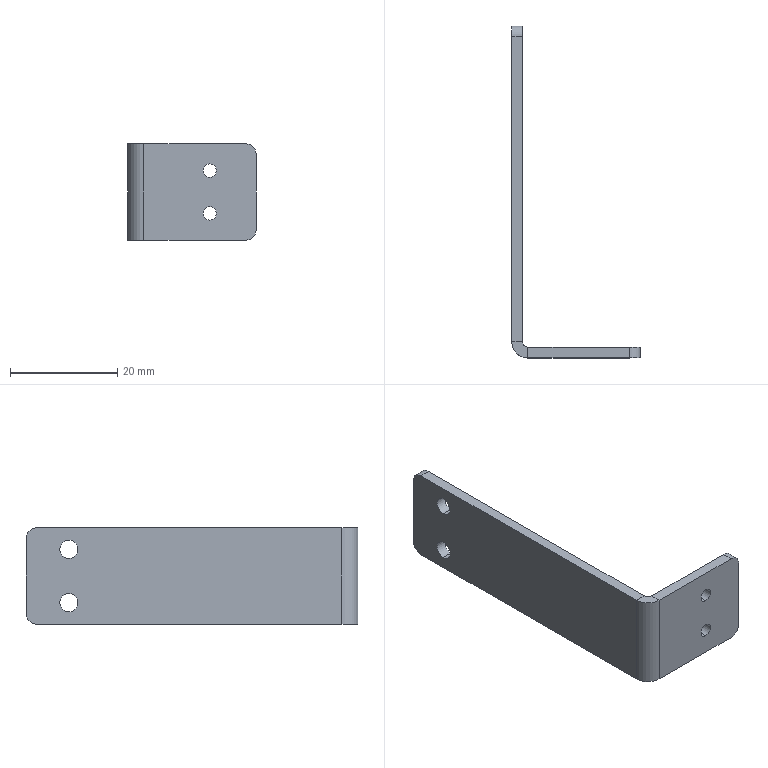Part | NX | features BREP 1 | 1 solid | 26 faces | box 24 x 62 x 18 mm | volume 2930 mm3 | cylinder 14 | plane 12 | commonest cylinder face diameters 2.5 x4 3.4 x4 4 x4 2 x1 6 x1
STEP:
#1=CARTESIAN_POINT('',(-2.,52.,6.7));
#2=VERTEX_POINT('',#1);
#3=CARTESIAN_POINT('',(0.,52.,6.7));
#4=VERTEX_POINT('',#3);
#5=CARTESIAN_POINT('',(0.,52.,6.7));
#6=DIRECTION('',(1.,0.,0.));
#7=VECTOR('',#6,1000.);
#8=LINE('',#5,#7);
#9=EDGE_CURVE('',#2,#4,#8,.T.);
#10=ORIENTED_EDGE('',*,*,#9,.F.);
#11=CARTESIAN_POINT('',(-2.,52.,3.3));
#12=VERTEX_POINT('',#11);
#13=CARTESIAN_POINT('',(-2.,52.,5.));
#14=DIRECTION('',(1.,0.,0.));
#15=DIRECTION('',(0.,0.,-1.));
#16=AXIS2_PLACEMENT_3D('',#13,#14,#15);
#17=CIRCLE('',#16,1.7);
#18=EDGE_CURVE('',#12,#2,#17,.T.);
#19=ORIENTED_EDGE('',*,*,#18,.F.);
#20=CARTESIAN_POINT('',(0.,52.,3.3));
#21=VERTEX_POINT('',#20);
#22=CARTESIAN_POINT('',(0.,52.,3.3));
#23=DIRECTION('',(1.,0.,0.));
#24=VECTOR('',#23,1000.);
#25=LINE('',#22,#24);
#26=EDGE_CURVE('',#12,#21,#25,.T.);
#27=ORIENTED_EDGE('',*,*,#26,.T.);
#28=CARTESIAN_POINT('',(0.,52.,5.));
#29=DIRECTION('',(1.,0.,0.));
#30=DIRECTION('',(0.,0.,-1.));
#31=AXIS2_PLACEMENT_3D('',#28,#29,#30);
#32=CIRCLE('',#31,1.7);
#33=EDGE_CURVE('',#21,#4,#32,.T.);
#34=ORIENTED_EDGE('',*,*,#33,.T.);
#35=EDGE_LOOP('',(#10,#19,#27,#34));
#36=FACE_BOUND('',#35,.T.);
#37=CARTESIAN_POINT('',(0.,52.,5.));
#38=DIRECTION('',(1.,0.,0.));
#39=DIRECTION('',(0.,0.,-1.));
#40=AXIS2_PLACEMENT_3D('',#37,#38,#39);
#41=CYLINDRICAL_SURFACE('',#40,1.7);
#42=ADVANCED_FACE('',(#36),#41,.F.);
#43=CARTESIAN_POINT('',(-2.,52.,-3.3));
#44=VERTEX_POINT('',#43);
#45=CARTESIAN_POINT('',(0.,52.,-3.3));
#46=VERTEX_POINT('',#45);
#47=CARTESIAN_POINT('',(0.,52.,-3.3));
#48=DIRECTION('',(1.,0.,0.));
#49=VECTOR('',#48,1000.);
#50=LINE('',#47,#49);
#51=EDGE_CURVE('',#44,#46,#50,.T.);
#52=ORIENTED_EDGE('',*,*,#51,.F.);
#53=CARTESIAN_POINT('',(-2.,52.,-6.7));
#54=VERTEX_POINT('',#53);
#55=CARTESIAN_POINT('',(-2.,52.,-5.));
#56=DIRECTION('',(1.,0.,0.));
#57=DIRECTION('',(0.,0.,-1.));
#58=AXIS2_PLACEMENT_3D('',#55,#56,#57);
#59=CIRCLE('',#58,1.7);
#60=EDGE_CURVE('',#54,#44,#59,.T.);
#61=ORIENTED_EDGE('',*,*,#60,.F.);
#62=CARTESIAN_POINT('',(0.,52.,-6.7));
#63=VERTEX_POINT('',#62);
#64=CARTESIAN_POINT('',(0.,52.,-6.7));
#65=DIRECTION('',(1.,0.,0.));
#66=VECTOR('',#65,1000.);
#67=LINE('',#64,#66);
#68=EDGE_CURVE('',#54,#63,#67,.T.);
#69=ORIENTED_EDGE('',*,*,#68,.T.);
#70=CARTESIAN_POINT('',(0.,52.,-5.));
#71=DIRECTION('',(1.,0.,0.));
#72=DIRECTION('',(0.,0.,-1.));
#73=AXIS2_PLACEMENT_3D('',#70,#71,#72);
#74=CIRCLE('',#73,1.7);
#75=EDGE_CURVE('',#63,#46,#74,.T.);
#76=ORIENTED_EDGE('',*,*,#75,.T.);
#77=EDGE_LOOP('',(#52,#61,#69,#76));
#78=FACE_BOUND('',#77,.T.);
#79=CARTESIAN_POINT('',(0.,52.,-5.));
#80=DIRECTION('',(1.,0.,0.));
#81=DIRECTION('',(0.,0.,-1.));
#82=AXIS2_PLACEMENT_3D('',#79,#80,#81);
#83=CYLINDRICAL_SURFACE('',#82,1.7);
#84=ADVANCED_FACE('',(#78),#83,.F.);
#85=CARTESIAN_POINT('',(13.3,0.,5.25));
#86=VERTEX_POINT('',#85);
#87=CARTESIAN_POINT('',(13.3,-2.,5.25));
#88=VERTEX_POINT('',#87);
#89=CARTESIAN_POINT('',(13.3,-2.,5.25));
#90=DIRECTION('',(0.,-1.,0.));
#91=VECTOR('',#90,1000.);
#92=LINE('',#89,#91);
#93=EDGE_CURVE('',#86,#88,#92,.T.);
#94=ORIENTED_EDGE('',*,*,#93,.F.);
#95=CARTESIAN_POINT('',(13.3,0.,2.75));
#96=VERTEX_POINT('',#95);
#97=CARTESIAN_POINT('',(13.3,0.,4.));
#98=DIRECTION('',(0.,1.,0.));
#99=DIRECTION('',(0.,0.,1.));
#100=AXIS2_PLACEMENT_3D('',#97,#98,#99);
#101=CIRCLE('',#100,1.25);
#102=EDGE_CURVE('',#86,#96,#101,.T.);
#103=ORIENTED_EDGE('',*,*,#102,.T.);
#104=CARTESIAN_POINT('',(13.3,-2.,2.75));
#105=VERTEX_POINT('',#104);
#106=CARTESIAN_POINT('',(13.3,-2.,2.75));
#107=DIRECTION('',(0.,-1.,0.));
#108=VECTOR('',#107,1000.);
#109=LINE('',#106,#108);
#110=EDGE_CURVE('',#96,#105,#109,.T.);
#111=ORIENTED_EDGE('',*,*,#110,.T.);
#112=CARTESIAN_POINT('',(13.3,-2.,4.));
#113=DIRECTION('',(0.,-1.,0.));
#114=DIRECTION('',(0.,0.,-1.));
#115=AXIS2_PLACEMENT_3D('',#112,#113,#114);
#116=CIRCLE('',#115,1.25);
#117=EDGE_CURVE('',#105,#88,#116,.T.);
#118=ORIENTED_EDGE('',*,*,#117,.T.);
#119=EDGE_LOOP('',(#94,#103,#111,#118));
#120=FACE_BOUND('',#119,.T.);
#121=CARTESIAN_POINT('',(13.3,-2.,4.));
#122=DIRECTION('',(0.,-1.,0.));
#123=DIRECTION('',(0.,0.,-1.));
#124=AXIS2_PLACEMENT_3D('',#121,#122,#123);
#125=CYLINDRICAL_SURFACE('',#124,1.25);
#126=ADVANCED_FACE('',(#120),#125,.F.);
#127=CARTESIAN_POINT('',(13.3,0.,-2.75));
#128=VERTEX_POINT('',#127);
#129=CARTESIAN_POINT('',(13.3,-2.,-2.75));
#130=VERTEX_POINT('',#129);
#131=CARTESIAN_POINT('',(13.3,-2.,-2.75));
#132=DIRECTION('',(0.,-1.,0.));
#133=VECTOR('',#132,1000.);
#134=LINE('',#131,#133);
#135=EDGE_CURVE('',#128,#130,#134,.T.);
#136=ORIENTED_EDGE('',*,*,#135,.F.);
#137=CARTESIAN_POINT('',(13.3,0.,-5.25));
#138=VERTEX_POINT('',#137);
#139=CARTESIAN_POINT('',(13.3,0.,-4.));
#140=DIRECTION('',(0.,1.,0.));
#141=DIRECTION('',(0.,0.,1.));
#142=AXIS2_PLACEMENT_3D('',#139,#140,#141);
#143=CIRCLE('',#142,1.25);
#144=EDGE_CURVE('',#128,#138,#143,.T.);
#145=ORIENTED_EDGE('',*,*,#144,.T.);
#146=CARTESIAN_POINT('',(13.3,-2.,-5.25));
#147=VERTEX_POINT('',#146);
#148=CARTESIAN_POINT('',(13.3,-2.,-5.25));
#149=DIRECTION('',(0.,-1.,0.));
#150=VECTOR('',#149,1000.);
#151=LINE('',#148,#150);
#152=EDGE_CURVE('',#138,#147,#151,.T.);
#153=ORIENTED_EDGE('',*,*,#152,.T.);
#154=CARTESIAN_POINT('',(13.3,-2.,-4.));
#155=DIRECTION('',(0.,-1.,0.));
#156=DIRECTION('',(0.,0.,-1.));
#157=AXIS2_PLACEMENT_3D('',#154,#155,#156);
#158=CIRCLE('',#157,1.25);
#159=EDGE_CURVE('',#147,#130,#158,.T.);
#160=ORIENTED_EDGE('',*,*,#159,.T.);
#161=EDGE_LOOP('',(#136,#145,#153,#160));
#162=FACE_BOUND('',#161,.T.);
#163=CARTESIAN_POINT('',(13.3,-2.,-4.));
#164=DIRECTION('',(0.,-1.,0.));
#165=DIRECTION('',(0.,0.,-1.));
#166=AXIS2_PLACEMENT_3D('',#163,#164,#165);
#167=CYLINDRICAL_SURFACE('',#166,1.25);
#168=ADVANCED_FACE('',(#162),#167,.F.);
#169=CARTESIAN_POINT('',(-2.,60.,-7.));
#170=VERTEX_POINT('',#169);
#171=CARTESIAN_POINT('',(-2.,58.,-9.));
#172=VERTEX_POINT('',#171);
#173=CARTESIAN_POINT('',(-2.,58.,-7.));
#174=DIRECTION('',(-1.,0.,0.));
#175=DIRECTION('',(0.,1.,0.));
#176=AXIS2_PLACEMENT_3D('',#173,#174,#175);
#177=CIRCLE('',#176,2.);
#178=EDGE_CURVE('',#170,#172,#177,.T.);
#179=ORIENTED_EDGE('',*,*,#178,.F.);
#180=CARTESIAN_POINT('',(0.,60.,-7.));
#181=VERTEX_POINT('',#180);
#182=CARTESIAN_POINT('',(-2.,60.,-7.));
#183=DIRECTION('',(-1.,0.,0.));
#184=VECTOR('',#183,1000.);
#185=LINE('',#182,#184);
#186=EDGE_CURVE('',#181,#170,#185,.T.);
#187=ORIENTED_EDGE('',*,*,#186,.F.);
#188=CARTESIAN_POINT('',(0.,58.,-9.));
#189=VERTEX_POINT('',#188);
#190=CARTESIAN_POINT('',(0.,58.,-7.));
#191=DIRECTION('',(1.,0.,0.));
#192=DIRECTION('',(0.,1.,0.));
#193=AXIS2_PLACEMENT_3D('',#190,#191,#192);
#194=CIRCLE('',#193,2.);
#195=EDGE_CURVE('',#189,#181,#194,.T.);
#196=ORIENTED_EDGE('',*,*,#195,.F.);
#197=CARTESIAN_POINT('',(1.,58.,-9.));
#198=DIRECTION('',(1.,0.,0.));
#199=VECTOR('',#198,1000.);
#200=LINE('',#197,#199);
#201=EDGE_CURVE('',#172,#189,#200,.T.);
#202=ORIENTED_EDGE('',*,*,#201,.F.);
#203=EDGE_LOOP('',(#179,#187,#196,#202));
#204=FACE_BOUND('',#203,.T.);
#205=CARTESIAN_POINT('',(1.,58.,-7.));
#206=DIRECTION('',(1.,0.,0.));
#207=DIRECTION('',(0.,0.,-1.));
#208=AXIS2_PLACEMENT_3D('',#205,#206,#207);
#209=CYLINDRICAL_SURFACE('',#208,2.);
#210=ADVANCED_FACE('',(#204),#209,.T.);
#211=CARTESIAN_POINT('',(-2.,58.,9.));
#212=VERTEX_POINT('',#211);
#213=CARTESIAN_POINT('',(-2.,60.,7.));
#214=VERTEX_POINT('',#213);
#215=CARTESIAN_POINT('',(-2.,58.,7.));
#216=DIRECTION('',(-1.,0.,0.));
#217=DIRECTION('',(0.,1.,0.));
#218=AXIS2_PLACEMENT_3D('',#215,#216,#217);
#219=CIRCLE('',#218,2.);
#220=EDGE_CURVE('',#212,#214,#219,.T.);
#221=ORIENTED_EDGE('',*,*,#220,.F.);
#222=CARTESIAN_POINT('',(0.,58.,9.));
#223=VERTEX_POINT('',#222);
#224=CARTESIAN_POINT('',(-2.,58.,9.));
#225=DIRECTION('',(-1.,0.,0.));
#226=VECTOR('',#225,1000.);
#227=LINE('',#224,#226);
#228=EDGE_CURVE('',#223,#212,#227,.T.);
#229=ORIENTED_EDGE('',*,*,#228,.F.);
#230=CARTESIAN_POINT('',(0.,60.,7.));
#231=VERTEX_POINT('',#230);
#232=CARTESIAN_POINT('',(0.,58.,7.));
#233=DIRECTION('',(1.,0.,0.));
#234=DIRECTION('',(0.,1.,0.));
#235=AXIS2_PLACEMENT_3D('',#232,#233,#234);
#236=CIRCLE('',#235,2.);
#237=EDGE_CURVE('',#231,#223,#236,.T.);
#238=ORIENTED_EDGE('',*,*,#237,.F.);
#239=CARTESIAN_POINT('',(0.,60.,7.));
#240=DIRECTION('',(1.,0.,0.));
#241=VECTOR('',#240,1000.);
#242=LINE('',#239,#241);
#243=EDGE_CURVE('',#214,#231,#242,.T.);
#244=ORIENTED_EDGE('',*,*,#243,.F.);
#245=EDGE_LOOP('',(#221,#229,#238,#244));
#246=FACE_BOUND('',#245,.T.);
#247=CARTESIAN_POINT('',(-2.,58.,7.));
#248=DIRECTION('',(-1.,0.,0.));
#249=DIRECTION('',(0.,0.,1.));
#250=AXIS2_PLACEMENT_3D('',#247,#248,#249);
#251=CYLINDRICAL_SURFACE('',#250,2.);
#252=ADVANCED_FACE('',(#246),#251,.T.);
#253=CARTESIAN_POINT('',(20.,0.,9.));
#254=VERTEX_POINT('',#253);
#255=CARTESIAN_POINT('',(22.,0.,7.));
#256=VERTEX_POINT('',#255);
#257=CARTESIAN_POINT('',(20.,0.,7.));
#258=DIRECTION('',(0.,1.,0.));
#259=DIRECTION('',(0.,0.,1.));
#260=AXIS2_PLACEMENT_3D('',#257,#258,#259);
#261=CIRCLE('',#260,2.);
#262=EDGE_CURVE('',#254,#256,#261,.T.);
#263=ORIENTED_EDGE('',*,*,#262,.F.);
#264=CARTESIAN_POINT('',(20.,-2.,9.));
#265=VERTEX_POINT('',#264);
#266=CARTESIAN_POINT('',(20.,1.,9.));
#267=DIRECTION('',(0.,1.,0.));
#268=VECTOR('',#267,1000.);
#269=LINE('',#266,#268);
#270=EDGE_CURVE('',#265,#254,#269,.T.);
#271=ORIENTED_EDGE('',*,*,#270,.F.);
#272=CARTESIAN_POINT('',(22.,-2.,7.));
#273=VERTEX_POINT('',#272);
#274=CARTESIAN_POINT('',(20.,-2.,7.));
#275=DIRECTION('',(0.,-1.,0.));
#276=DIRECTION('',(0.,0.,1.));
#277=AXIS2_PLACEMENT_3D('',#274,#275,#276);
#278=CIRCLE('',#277,2.);
#279=EDGE_CURVE('',#273,#265,#278,.T.);
#280=ORIENTED_EDGE('',*,*,#279,.F.);
#281=CARTESIAN_POINT('',(22.,0.,7.));
#282=DIRECTION('',(0.,-1.,0.));
#283=VECTOR('',#282,1000.);
#284=LINE('',#281,#283);
#285=EDGE_CURVE('',#256,#273,#284,.T.);
#286=ORIENTED_EDGE('',*,*,#285,.F.);
#287=EDGE_LOOP('',(#263,#271,#280,#286));
#288=FACE_BOUND('',#287,.T.);
#289=CARTESIAN_POINT('',(20.,0.,7.));
#290=DIRECTION('',(0.,-1.,0.));
#291=DIRECTION('',(0.,0.,-1.));
#292=AXIS2_PLACEMENT_3D('',#289,#290,#291);
#293=CYLINDRICAL_SURFACE('',#292,2.);
#294=ADVANCED_FACE('',(#288),#293,.T.);
#295=CARTESIAN_POINT('',(22.,0.,-7.));
#296=VERTEX_POINT('',#295);
#297=CARTESIAN_POINT('',(20.,0.,-9.));
#298=VERTEX_POINT('',#297);
#299=CARTESIAN_POINT('',(20.,0.,-7.));
#300=DIRECTION('',(0.,1.,0.));
#301=DIRECTION('',(0.,0.,1.));
#302=AXIS2_PLACEMENT_3D('',#299,#300,#301);
#303=CIRCLE('',#302,2.);
#304=EDGE_CURVE('',#296,#298,#303,.T.);
#305=ORIENTED_EDGE('',*,*,#304,.F.);
#306=CARTESIAN_POINT('',(22.,-2.,-7.));
#307=VERTEX_POINT('',#306);
#308=CARTESIAN_POINT('',(22.,0.,-7.));
#309=DIRECTION('',(0.,1.,0.));
#310=VECTOR('',#309,1000.);
#311=LINE('',#308,#310);
#312=EDGE_CURVE('',#307,#296,#311,.T.);
#313=ORIENTED_EDGE('',*,*,#312,.F.);
#314=CARTESIAN_POINT('',(20.,-2.,-9.));
#315=VERTEX_POINT('',#314);
#316=CARTESIAN_POINT('',(20.,-2.,-7.));
#317=DIRECTION('',(0.,-1.,0.));
#318=DIRECTION('',(0.,0.,1.));
#319=AXIS2_PLACEMENT_3D('',#316,#317,#318);
#320=CIRCLE('',#319,2.);
#321=EDGE_CURVE('',#315,#307,#320,.T.);
#322=ORIENTED_EDGE('',*,*,#321,.F.);
#323=CARTESIAN_POINT('',(20.,1.,-9.));
#324=DIRECTION('',(0.,-1.,0.));
#325=VECTOR('',#324,1000.);
#326=LINE('',#323,#325);
#327=EDGE_CURVE('',#298,#315,#326,.T.);
#328=ORIENTED_EDGE('',*,*,#327,.F.);
#329=EDGE_LOOP('',(#305,#313,#322,#328));
#330=FACE_BOUND('',#329,.T.);
#331=CARTESIAN_POINT('',(20.,1.,-7.));
#332=DIRECTION('',(0.,-1.,0.));
#333=DIRECTION('',(0.,0.,-1.));
#334=AXIS2_PLACEMENT_3D('',#331,#332,#333);
#335=CYLINDRICAL_SURFACE('',#334,2.);
#336=ADVANCED_FACE('',(#330),#335,.T.);
#337=CARTESIAN_POINT('',(1.,0.,-9.));
#338=VERTEX_POINT('',#337);
#339=CARTESIAN_POINT('',(0.,0.,-9.));
#340=DIRECTION('',(1.,0.,0.));
#341=VECTOR('',#340,1000.);
#342=LINE('',#339,#341);
#343=EDGE_CURVE('',#338,#298,#342,.T.);
#344=ORIENTED_EDGE('',*,*,#343,.T.);
#345=ORIENTED_EDGE('',*,*,#327,.T.);
#346=CARTESIAN_POINT('',(1.,-2.,-9.));
#347=VERTEX_POINT('',#346);
#348=CARTESIAN_POINT('',(0.,-2.,-9.));
#349=DIRECTION('',(1.,0.,0.));
#350=VECTOR('',#349,1000.);
#351=LINE('',#348,#350);
#352=EDGE_CURVE('',#347,#315,#351,.T.);
#353=ORIENTED_EDGE('',*,*,#352,.F.);
#354=CARTESIAN_POINT('',(1.,-2.,-9.));
#355=DIRECTION('',(0.,1.,0.));
#356=VECTOR('',#355,1000.);
#357=LINE('',#354,#356);
#358=EDGE_CURVE('',#347,#338,#357,.T.);
#359=ORIENTED_EDGE('',*,*,#358,.T.);
#360=EDGE_LOOP('',(#344,#345,#353,#359));
#361=FACE_BOUND('',#360,.T.);
#362=CARTESIAN_POINT('',(1.,1.,-9.));
#363=DIRECTION('',(0.,0.,-1.));
#364=DIRECTION('',(-1.,0.,0.));
#365=AXIS2_PLACEMENT_3D('',#362,#363,#364);
#366=PLANE('',#365);
#367=ADVANCED_FACE('',(#361),#366,.T.);
#368=CARTESIAN_POINT('',(0.,1.,9.));
#369=VERTEX_POINT('',#368);
#370=CARTESIAN_POINT('',(0.,60.,9.));
#371=DIRECTION('',(0.,-1.,0.));
#372=VECTOR('',#371,1000.);
#373=LINE('',#370,#372);
#374=EDGE_CURVE('',#223,#369,#373,.T.);
#375=ORIENTED_EDGE('',*,*,#374,.F.);
#376=ORIENTED_EDGE('',*,*,#228,.T.);
#377=CARTESIAN_POINT('',(-2.,1.,9.));
#378=VERTEX_POINT('',#377);
#379=CARTESIAN_POINT('',(-2.,60.,9.));
#380=DIRECTION('',(0.,-1.,0.));
#381=VECTOR('',#380,1000.);
#382=LINE('',#379,#381);
#383=EDGE_CURVE('',#212,#378,#382,.T.);
#384=ORIENTED_EDGE('',*,*,#383,.T.);
#385=CARTESIAN_POINT('',(-2.,1.,9.));
#386=DIRECTION('',(1.,0.,0.));
#387=VECTOR('',#386,1000.);
#388=LINE('',#385,#387);
#389=EDGE_CURVE('',#378,#369,#388,.T.);
#390=ORIENTED_EDGE('',*,*,#389,.T.);
#391=EDGE_LOOP('',(#375,#376,#384,#390));
#392=FACE_BOUND('',#391,.T.);
#393=CARTESIAN_POINT('',(1.,1.,9.));
#394=DIRECTION('',(0.,0.,-1.));
#395=DIRECTION('',(-1.,0.,0.));
#396=AXIS2_PLACEMENT_3D('',#393,#394,#395);
#397=PLANE('',#396);
#398=ADVANCED_FACE('',(#392),#397,.F.);
#399=CARTESIAN_POINT('',(-2.,1.,-9.));
#400=VERTEX_POINT('',#399);
#401=CARTESIAN_POINT('',(1.,1.,-9.));
#402=DIRECTION('',(0.,0.,1.));
#403=DIRECTION('',(1.,0.,0.));
#404=AXIS2_PLACEMENT_3D('',#401,#402,#403);
#405=CIRCLE('',#404,3.);
#406=EDGE_CURVE('',#400,#347,#405,.T.);
#407=ORIENTED_EDGE('',*,*,#406,.T.);
#408=CARTESIAN_POINT('',(1.,-2.,9.));
#409=VERTEX_POINT('',#408);
#410=CARTESIAN_POINT('',(1.,-2.,9.));
#411=DIRECTION('',(0.,0.,-1.));
#412=VECTOR('',#411,1000.);
#413=LINE('',#410,#412);
#414=EDGE_CURVE('',#409,#347,#413,.T.);
#415=ORIENTED_EDGE('',*,*,#414,.F.);
#416=CARTESIAN_POINT('',(1.,1.,9.));
#417=DIRECTION('',(0.,0.,1.));
#418=DIRECTION('',(1.,0.,0.));
#419=AXIS2_PLACEMENT_3D('',#416,#417,#418);
#420=CIRCLE('',#419,3.);
#421=EDGE_CURVE('',#378,#409,#420,.T.);
#422=ORIENTED_EDGE('',*,*,#421,.F.);
#423=CARTESIAN_POINT('',(-2.,1.,9.));
#424=DIRECTION('',(0.,0.,-1.));
#425=VECTOR('',#424,1000.);
#426=LINE('',#423,#425);
#427=EDGE_CURVE('',#378,#400,#426,.T.);
#428=ORIENTED_EDGE('',*,*,#427,.T.);
#429=EDGE_LOOP('',(#407,#415,#422,#428));
#430=FACE_BOUND('',#429,.T.);
#431=CARTESIAN_POINT('',(1.,1.,9.));
#432=DIRECTION('',(0.,0.,-1.));
#433=DIRECTION('',(-1.,0.,0.));
#434=AXIS2_PLACEMENT_3D('',#431,#432,#433);
#435=CYLINDRICAL_SURFACE('',#434,3.);
#436=ADVANCED_FACE('',(#430),#435,.T.);
#437=ORIENTED_EDGE('',*,*,#383,.F.);
#438=ORIENTED_EDGE('',*,*,#220,.T.);
#439=CARTESIAN_POINT('',(-2.,60.,9.));
#440=DIRECTION('',(0.,0.,-1.));
#441=VECTOR('',#440,1000.);
#442=LINE('',#439,#441);
#443=EDGE_CURVE('',#214,#170,#442,.T.);
#444=ORIENTED_EDGE('',*,*,#443,.T.);
#445=ORIENTED_EDGE('',*,*,#178,.T.);
#446=CARTESIAN_POINT('',(-2.,60.,-9.));
#447=DIRECTION('',(0.,-1.,0.));
#448=VECTOR('',#447,1000.);
#449=LINE('',#446,#448);
#450=EDGE_CURVE('',#172,#400,#449,.T.);
#451=ORIENTED_EDGE('',*,*,#450,.T.);
#452=ORIENTED_EDGE('',*,*,#427,.F.);
#453=EDGE_LOOP('',(#437,#438,#444,#445,#451,#452));
#454=FACE_BOUND('',#453,.T.);
#455=ORIENTED_EDGE('',*,*,#60,.T.);
#456=CARTESIAN_POINT('',(-2.,52.,-5.));
#457=DIRECTION('',(1.,0.,0.));
#458=DIRECTION('',(0.,0.,-1.));
#459=AXIS2_PLACEMENT_3D('',#456,#457,#458);
#460=CIRCLE('',#459,1.7);
#461=EDGE_CURVE('',#44,#54,#460,.T.);
#462=ORIENTED_EDGE('',*,*,#461,.T.);
#463=EDGE_LOOP('',(#455,#462));
#464=FACE_BOUND('',#463,.T.);
#465=ORIENTED_EDGE('',*,*,#18,.T.);
#466=CARTESIAN_POINT('',(-2.,52.,5.));
#467=DIRECTION('',(1.,0.,0.));
#468=DIRECTION('',(0.,0.,-1.));
#469=AXIS2_PLACEMENT_3D('',#466,#467,#468);
#470=CIRCLE('',#469,1.7);
#471=EDGE_CURVE('',#2,#12,#470,.T.);
#472=ORIENTED_EDGE('',*,*,#471,.T.);
#473=EDGE_LOOP('',(#465,#472));
#474=FACE_BOUND('',#473,.T.);
#475=CARTESIAN_POINT('',(-2.,60.,9.));
#476=DIRECTION('',(1.,0.,0.));
#477=DIRECTION('',(0.,1.,0.));
#478=AXIS2_PLACEMENT_3D('',#475,#476,#477);
#479=PLANE('',#478);
#480=ADVANCED_FACE('',(#454,#464,#474),#479,.F.);
#481=ORIENTED_EDGE('',*,*,#443,.F.);
#482=ORIENTED_EDGE('',*,*,#243,.T.);
#483=CARTESIAN_POINT('',(0.,60.,9.));
#484=DIRECTION('',(0.,0.,-1.));
#485=VECTOR('',#484,1000.);
#486=LINE('',#483,#485);
#487=EDGE_CURVE('',#231,#181,#486,.T.);
#488=ORIENTED_EDGE('',*,*,#487,.T.);
#489=ORIENTED_EDGE('',*,*,#186,.T.);
#490=EDGE_LOOP('',(#481,#482,#488,#489));
#491=FACE_BOUND('',#490,.T.);
#492=CARTESIAN_POINT('',(-2.,60.,9.));
#493=DIRECTION('',(0.,1.,0.));
#494=DIRECTION('',(0.,0.,1.));
#495=AXIS2_PLACEMENT_3D('',#492,#493,#494);
#496=PLANE('',#495);
#497=ADVANCED_FACE('',(#491),#496,.T.);
#498=ORIENTED_EDGE('',*,*,#487,.F.);
#499=ORIENTED_EDGE('',*,*,#237,.T.);
#500=ORIENTED_EDGE('',*,*,#374,.T.);
#501=CARTESIAN_POINT('',(0.,1.,-9.));
#502=VERTEX_POINT('',#501);
#503=CARTESIAN_POINT('',(0.,1.,9.));
#504=DIRECTION('',(0.,0.,-1.));
#505=VECTOR('',#504,1000.);
#506=LINE('',#503,#505);
#507=EDGE_CURVE('',#369,#502,#506,.T.);
#508=ORIENTED_EDGE('',*,*,#507,.T.);
#509=CARTESIAN_POINT('',(0.,60.,-9.));
#510=DIRECTION('',(0.,-1.,0.));
#511=VECTOR('',#510,1000.);
#512=LINE('',#509,#511);
#513=EDGE_CURVE('',#189,#502,#512,.T.);
#514=ORIENTED_EDGE('',*,*,#513,.F.);
#515=ORIENTED_EDGE('',*,*,#195,.T.);
#516=EDGE_LOOP('',(#498,#499,#500,#508,#514,#515));
#517=FACE_BOUND('',#516,.T.);
#518=ORIENTED_EDGE('',*,*,#75,.F.);
#519=CARTESIAN_POINT('',(0.,52.,-5.));
#520=DIRECTION('',(1.,0.,0.));
#521=DIRECTION('',(0.,0.,-1.));
#522=AXIS2_PLACEMENT_3D('',#519,#520,#521);
#523=CIRCLE('',#522,1.7);
#524=EDGE_CURVE('',#46,#63,#523,.T.);
#525=ORIENTED_EDGE('',*,*,#524,.F.);
#526=EDGE_LOOP('',(#518,#525));
#527=FACE_BOUND('',#526,.T.);
#528=ORIENTED_EDGE('',*,*,#33,.F.);
#529=CARTESIAN_POINT('',(0.,52.,5.));
#530=DIRECTION('',(1.,0.,0.));
#531=DIRECTION('',(0.,0.,-1.));
#532=AXIS2_PLACEMENT_3D('',#529,#530,#531);
#533=CIRCLE('',#532,1.7);
#534=EDGE_CURVE('',#4,#21,#533,.T.);
#535=ORIENTED_EDGE('',*,*,#534,.F.);
#536=EDGE_LOOP('',(#528,#535));
#537=FACE_BOUND('',#536,.T.);
#538=CARTESIAN_POINT('',(0.,60.,9.));
#539=DIRECTION('',(1.,0.,0.));
#540=DIRECTION('',(0.,1.,0.));
#541=AXIS2_PLACEMENT_3D('',#538,#539,#540);
#542=PLANE('',#541);
#543=ADVANCED_FACE('',(#517,#527,#537),#542,.T.);
#544=CARTESIAN_POINT('',(1.,1.,-9.));
#545=DIRECTION('',(0.,0.,1.));
#546=DIRECTION('',(-1.,0.,0.));
#547=AXIS2_PLACEMENT_3D('',#544,#545,#546);
#548=CIRCLE('',#547,1.);
#549=EDGE_CURVE('',#502,#338,#548,.T.);
#550=ORIENTED_EDGE('',*,*,#549,.F.);
#551=ORIENTED_EDGE('',*,*,#507,.F.);
#552=CARTESIAN_POINT('',(1.,0.,9.));
#553=VERTEX_POINT('',#552);
#554=CARTESIAN_POINT('',(1.,1.,9.));
#555=DIRECTION('',(0.,0.,1.));
#556=DIRECTION('',(-1.,0.,0.));
#557=AXIS2_PLACEMENT_3D('',#554,#555,#556);
#558=CIRCLE('',#557,1.);
#559=EDGE_CURVE('',#369,#553,#558,.T.);
#560=ORIENTED_EDGE('',*,*,#559,.T.);
#561=CARTESIAN_POINT('',(1.,0.,9.));
#562=DIRECTION('',(0.,0.,-1.));
#563=VECTOR('',#562,1000.);
#564=LINE('',#561,#563);
#565=EDGE_CURVE('',#553,#338,#564,.T.);
#566=ORIENTED_EDGE('',*,*,#565,.T.);
#567=EDGE_LOOP('',(#550,#551,#560,#566));
#568=FACE_BOUND('',#567,.T.);
#569=CARTESIAN_POINT('',(1.,1.,9.));
#570=DIRECTION('',(0.,0.,-1.));
#571=DIRECTION('',(-1.,0.,0.));
#572=AXIS2_PLACEMENT_3D('',#569,#570,#571);
#573=CYLINDRICAL_SURFACE('',#572,1.);
#574=ADVANCED_FACE('',(#568),#573,.F.);
#575=CARTESIAN_POINT('',(22.,0.,9.));
#576=DIRECTION('',(0.,0.,-1.));
#577=VECTOR('',#576,1000.);
#578=LINE('',#575,#577);
#579=EDGE_CURVE('',#256,#296,#578,.T.);
#580=ORIENTED_EDGE('',*,*,#579,.T.);
#581=ORIENTED_EDGE('',*,*,#304,.T.);
#582=ORIENTED_EDGE('',*,*,#343,.F.);
#583=ORIENTED_EDGE('',*,*,#565,.F.);
#584=CARTESIAN_POINT('',(0.,0.,9.));
#585=DIRECTION('',(1.,0.,0.));
#586=VECTOR('',#585,1000.);
#587=LINE('',#584,#586);
#588=EDGE_CURVE('',#553,#254,#587,.T.);
#589=ORIENTED_EDGE('',*,*,#588,.T.);
#590=ORIENTED_EDGE('',*,*,#262,.T.);
#591=EDGE_LOOP('',(#580,#581,#582,#583,#589,#590));
#592=FACE_BOUND('',#591,.T.);
#593=CARTESIAN_POINT('',(13.3,0.,-4.));
#594=DIRECTION('',(0.,1.,0.));
#595=DIRECTION('',(0.,0.,1.));
#596=AXIS2_PLACEMENT_3D('',#593,#594,#595);
#597=CIRCLE('',#596,1.25);
#598=EDGE_CURVE('',#138,#128,#597,.T.);
#599=ORIENTED_EDGE('',*,*,#598,.F.);
#600=ORIENTED_EDGE('',*,*,#144,.F.);
#601=EDGE_LOOP('',(#599,#600));
#602=FACE_BOUND('',#601,.T.);
#603=CARTESIAN_POINT('',(13.3,0.,4.));
#604=DIRECTION('',(0.,1.,0.));
#605=DIRECTION('',(0.,0.,1.));
#606=AXIS2_PLACEMENT_3D('',#603,#604,#605);
#607=CIRCLE('',#606,1.25);
#608=EDGE_CURVE('',#96,#86,#607,.T.);
#609=ORIENTED_EDGE('',*,*,#608,.F.);
#610=ORIENTED_EDGE('',*,*,#102,.F.);
#611=EDGE_LOOP('',(#609,#610));
#612=FACE_BOUND('',#611,.T.);
#613=CARTESIAN_POINT('',(0.,0.,9.));
#614=DIRECTION('',(0.,1.,0.));
#615=DIRECTION('',(0.,0.,1.));
#616=AXIS2_PLACEMENT_3D('',#613,#614,#615);
#617=PLANE('',#616);
#618=ADVANCED_FACE('',(#592,#602,#612),#617,.T.);
#619=CARTESIAN_POINT('',(22.,-2.,9.));
#620=DIRECTION('',(0.,0.,-1.));
#621=VECTOR('',#620,1000.);
#622=LINE('',#619,#621);
#623=EDGE_CURVE('',#273,#307,#622,.T.);
#624=ORIENTED_EDGE('',*,*,#623,.T.);
#625=ORIENTED_EDGE('',*,*,#312,.T.);
#626=ORIENTED_EDGE('',*,*,#579,.F.);
#627=ORIENTED_EDGE('',*,*,#285,.T.);
#628=EDGE_LOOP('',(#624,#625,#626,#627));
#629=FACE_BOUND('',#628,.T.);
#630=CARTESIAN_POINT('',(22.,0.,9.));
#631=DIRECTION('',(1.,0.,0.));
#632=DIRECTION('',(0.,0.,-1.));
#633=AXIS2_PLACEMENT_3D('',#630,#631,#632);
#634=PLANE('',#633);
#635=ADVANCED_FACE('',(#629),#634,.T.);
#636=ORIENTED_EDGE('',*,*,#352,.T.);
#637=ORIENTED_EDGE('',*,*,#321,.T.);
#638=ORIENTED_EDGE('',*,*,#623,.F.);
#639=ORIENTED_EDGE('',*,*,#279,.T.);
#640=CARTESIAN_POINT('',(0.,-2.,9.));
#641=DIRECTION('',(1.,0.,0.));
#642=VECTOR('',#641,1000.);
#643=LINE('',#640,#642);
#644=EDGE_CURVE('',#409,#265,#643,.T.);
#645=ORIENTED_EDGE('',*,*,#644,.F.);
#646=ORIENTED_EDGE('',*,*,#414,.T.);
#647=EDGE_LOOP('',(#636,#637,#638,#639,#645,#646));
#648=FACE_BOUND('',#647,.T.);
#649=ORIENTED_EDGE('',*,*,#159,.F.);
#650=CARTESIAN_POINT('',(13.3,-2.,-4.));
#651=DIRECTION('',(0.,-1.,0.));
#652=DIRECTION('',(0.,0.,-1.));
#653=AXIS2_PLACEMENT_3D('',#650,#651,#652);
#654=CIRCLE('',#653,1.25);
#655=EDGE_CURVE('',#130,#147,#654,.T.);
#656=ORIENTED_EDGE('',*,*,#655,.F.);
#657=EDGE_LOOP('',(#649,#656));
#658=FACE_BOUND('',#657,.T.);
#659=ORIENTED_EDGE('',*,*,#117,.F.);
#660=CARTESIAN_POINT('',(13.3,-2.,4.));
#661=DIRECTION('',(0.,-1.,0.));
#662=DIRECTION('',(0.,0.,-1.));
#663=AXIS2_PLACEMENT_3D('',#660,#661,#662);
#664=CIRCLE('',#663,1.25);
#665=EDGE_CURVE('',#88,#105,#664,.T.);
#666=ORIENTED_EDGE('',*,*,#665,.F.);
#667=EDGE_LOOP('',(#659,#666));
#668=FACE_BOUND('',#667,.T.);
#669=CARTESIAN_POINT('',(0.,-2.,9.));
#670=DIRECTION('',(0.,1.,0.));
#671=DIRECTION('',(0.,0.,1.));
#672=AXIS2_PLACEMENT_3D('',#669,#670,#671);
#673=PLANE('',#672);
#674=ADVANCED_FACE('',(#648,#658,#668),#673,.F.);
#675=ORIENTED_EDGE('',*,*,#450,.F.);
#676=ORIENTED_EDGE('',*,*,#201,.T.);
#677=ORIENTED_EDGE('',*,*,#513,.T.);
#678=CARTESIAN_POINT('',(0.,1.,-9.));
#679=DIRECTION('',(-1.,0.,0.));
#680=VECTOR('',#679,1000.);
#681=LINE('',#678,#680);
#682=EDGE_CURVE('',#502,#400,#681,.T.);
#683=ORIENTED_EDGE('',*,*,#682,.T.);
#684=EDGE_LOOP('',(#675,#676,#677,#683));
#685=FACE_BOUND('',#684,.T.);
#686=CARTESIAN_POINT('',(1.,-2.,-9.));
#687=DIRECTION('',(0.,0.,-1.));
#688=DIRECTION('',(-1.,0.,0.));
#689=AXIS2_PLACEMENT_3D('',#686,#687,#688);
#690=PLANE('',#689);
#691=ADVANCED_FACE('',(#685),#690,.T.);
#692=ORIENTED_EDGE('',*,*,#682,.F.);
#693=ORIENTED_EDGE('',*,*,#549,.T.);
#694=ORIENTED_EDGE('',*,*,#358,.F.);
#695=ORIENTED_EDGE('',*,*,#406,.F.);
#696=EDGE_LOOP('',(#692,#693,#694,#695));
#697=FACE_BOUND('',#696,.T.);
#698=CARTESIAN_POINT('',(0.,1.,-9.));
#699=DIRECTION('',(0.,0.,-1.));
#700=DIRECTION('',(-1.,0.,0.));
#701=AXIS2_PLACEMENT_3D('',#698,#699,#700);
#702=PLANE('',#701);
#703=ADVANCED_FACE('',(#697),#702,.T.);
#704=ORIENTED_EDGE('',*,*,#644,.T.);
#705=ORIENTED_EDGE('',*,*,#270,.T.);
#706=ORIENTED_EDGE('',*,*,#588,.F.);
#707=CARTESIAN_POINT('',(1.,0.,9.));
#708=DIRECTION('',(0.,-1.,0.));
#709=VECTOR('',#708,1000.);
#710=LINE('',#707,#709);
#711=EDGE_CURVE('',#553,#409,#710,.T.);
#712=ORIENTED_EDGE('',*,*,#711,.T.);
#713=EDGE_LOOP('',(#704,#705,#706,#712));
#714=FACE_BOUND('',#713,.T.);
#715=CARTESIAN_POINT('',(-2.,1.,9.));
#716=DIRECTION('',(0.,0.,1.));
#717=DIRECTION('',(1.,0.,0.));
#718=AXIS2_PLACEMENT_3D('',#715,#716,#717);
#719=PLANE('',#718);
#720=ADVANCED_FACE('',(#714),#719,.T.);
#721=ORIENTED_EDGE('',*,*,#711,.F.);
#722=ORIENTED_EDGE('',*,*,#559,.F.);
#723=ORIENTED_EDGE('',*,*,#389,.F.);
#724=ORIENTED_EDGE('',*,*,#421,.T.);
#725=EDGE_LOOP('',(#721,#722,#723,#724));
#726=FACE_BOUND('',#725,.T.);
#727=CARTESIAN_POINT('',(1.,0.,9.));
#728=DIRECTION('',(0.,0.,1.));
#729=DIRECTION('',(1.,0.,0.));
#730=AXIS2_PLACEMENT_3D('',#727,#728,#729);
#731=PLANE('',#730);
#732=ADVANCED_FACE('',(#726),#731,.T.);
#733=ORIENTED_EDGE('',*,*,#598,.T.);
#734=ORIENTED_EDGE('',*,*,#135,.T.);
#735=ORIENTED_EDGE('',*,*,#655,.T.);
#736=ORIENTED_EDGE('',*,*,#152,.F.);
#737=EDGE_LOOP('',(#733,#734,#735,#736));
#738=FACE_BOUND('',#737,.T.);
#739=CARTESIAN_POINT('',(13.3,-2.,-4.));
#740=DIRECTION('',(0.,-1.,0.));
#741=DIRECTION('',(0.,0.,-1.));
#742=AXIS2_PLACEMENT_3D('',#739,#740,#741);
#743=CYLINDRICAL_SURFACE('',#742,1.25);
#744=ADVANCED_FACE('',(#738),#743,.F.);
#745=ORIENTED_EDGE('',*,*,#608,.T.);
#746=ORIENTED_EDGE('',*,*,#93,.T.);
#747=ORIENTED_EDGE('',*,*,#665,.T.);
#748=ORIENTED_EDGE('',*,*,#110,.F.);
#749=EDGE_LOOP('',(#745,#746,#747,#748));
#750=FACE_BOUND('',#749,.T.);
#751=CARTESIAN_POINT('',(13.3,-2.,4.));
#752=DIRECTION('',(0.,-1.,0.));
#753=DIRECTION('',(0.,0.,-1.));
#754=AXIS2_PLACEMENT_3D('',#751,#752,#753);
#755=CYLINDRICAL_SURFACE('',#754,1.25);
#756=ADVANCED_FACE('',(#750),#755,.F.);
#757=ORIENTED_EDGE('',*,*,#461,.F.);
#758=ORIENTED_EDGE('',*,*,#51,.T.);
#759=ORIENTED_EDGE('',*,*,#524,.T.);
#760=ORIENTED_EDGE('',*,*,#68,.F.);
#761=EDGE_LOOP('',(#757,#758,#759,#760));
#762=FACE_BOUND('',#761,.T.);
#763=CARTESIAN_POINT('',(0.,52.,-5.));
#764=DIRECTION('',(1.,0.,0.));
#765=DIRECTION('',(0.,0.,-1.));
#766=AXIS2_PLACEMENT_3D('',#763,#764,#765);
#767=CYLINDRICAL_SURFACE('',#766,1.7);
#768=ADVANCED_FACE('',(#762),#767,.F.);
#769=ORIENTED_EDGE('',*,*,#471,.F.);
#770=ORIENTED_EDGE('',*,*,#9,.T.);
#771=ORIENTED_EDGE('',*,*,#534,.T.);
#772=ORIENTED_EDGE('',*,*,#26,.F.);
#773=EDGE_LOOP('',(#769,#770,#771,#772));
#774=FACE_BOUND('',#773,.T.);
#775=CARTESIAN_POINT('',(0.,52.,5.));
#776=DIRECTION('',(1.,0.,0.));
#777=DIRECTION('',(0.,0.,-1.));
#778=AXIS2_PLACEMENT_3D('',#775,#776,#777);
#779=CYLINDRICAL_SURFACE('',#778,1.7);
#780=ADVANCED_FACE('',(#774),#779,.F.);
#781=CLOSED_SHELL('',(#42,#84,#126,#168,#210,#252,#294,#336,#367,#398,#436,#480,#497,#543,#574,#618,#635,#674,#691,#703,#720,#732,#744,#756,#768,#780));
#782=MANIFOLD_SOLID_BREP('',#781);
#783=(LENGTH_UNIT()NAMED_UNIT(*)SI_UNIT(.MILLI.,.METRE.));
#784=UNCERTAINTY_MEASURE_WITH_UNIT(LENGTH_MEASURE(0.00001),#783,'','');
#785=(NAMED_UNIT(*)PLANE_ANGLE_UNIT()SI_UNIT($,.RADIAN.));
#786=(NAMED_UNIT(*)SI_UNIT($,.STERADIAN.)SOLID_ANGLE_UNIT());
#787=(GEOMETRIC_REPRESENTATION_CONTEXT(3)GLOBAL_UNCERTAINTY_ASSIGNED_CONTEXT((#784))GLOBAL_UNIT_ASSIGNED_CONTEXT((#783,#785,#786))REPRESENTATION_CONTEXT('',''));
#788=ADVANCED_BREP_SHAPE_REPRESENTATION('',(#782),#787);